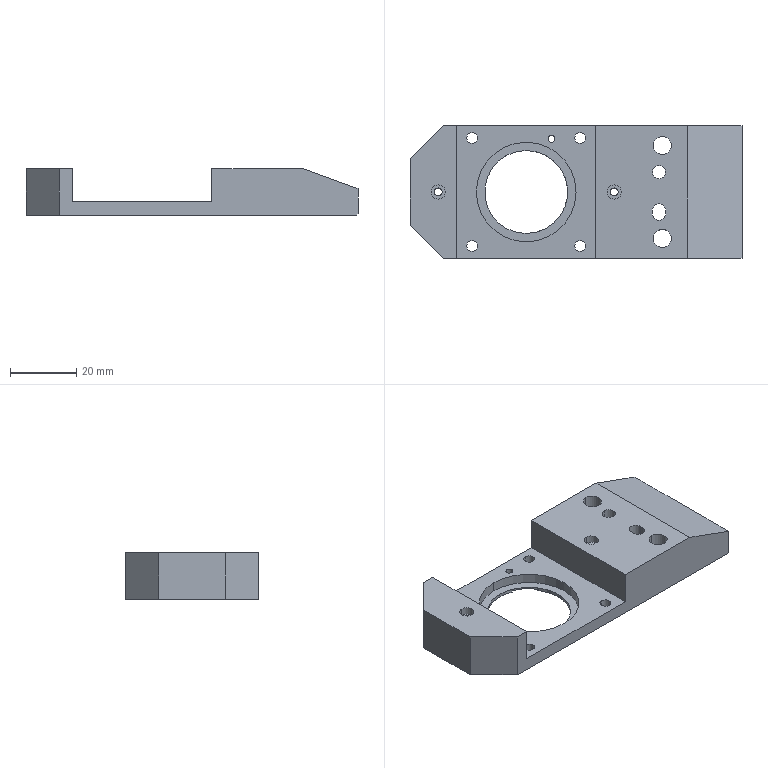Part | 1 solid | 71 faces | box 100 x 40 x 14 mm | volume 30710 mm3 | cylinder 43 | plane 28 | commonest cylinder face diameters 4 x9 3.3 x8 2.4 x4 4.3 x4 5.5 x4 7 x4